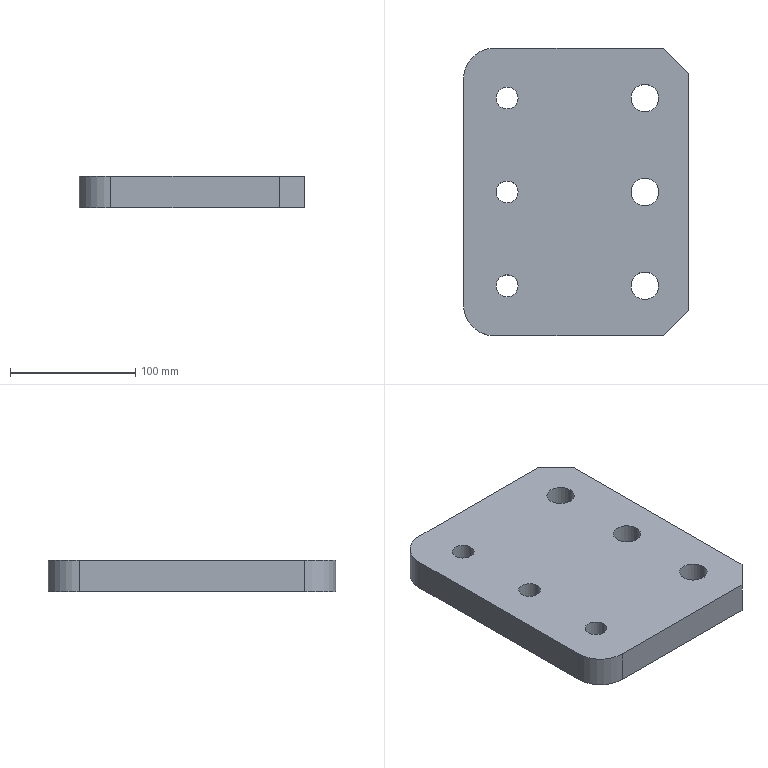Part | STEP file | 01-Connecting plate 1 | 1 solid | 22 faces | box 180 x 230 x 25 mm | volume 971744 mm3 | cylinder 14 | plane 8 | commonest cylinder face diameters 17.5 x6 22 x6 50 x2